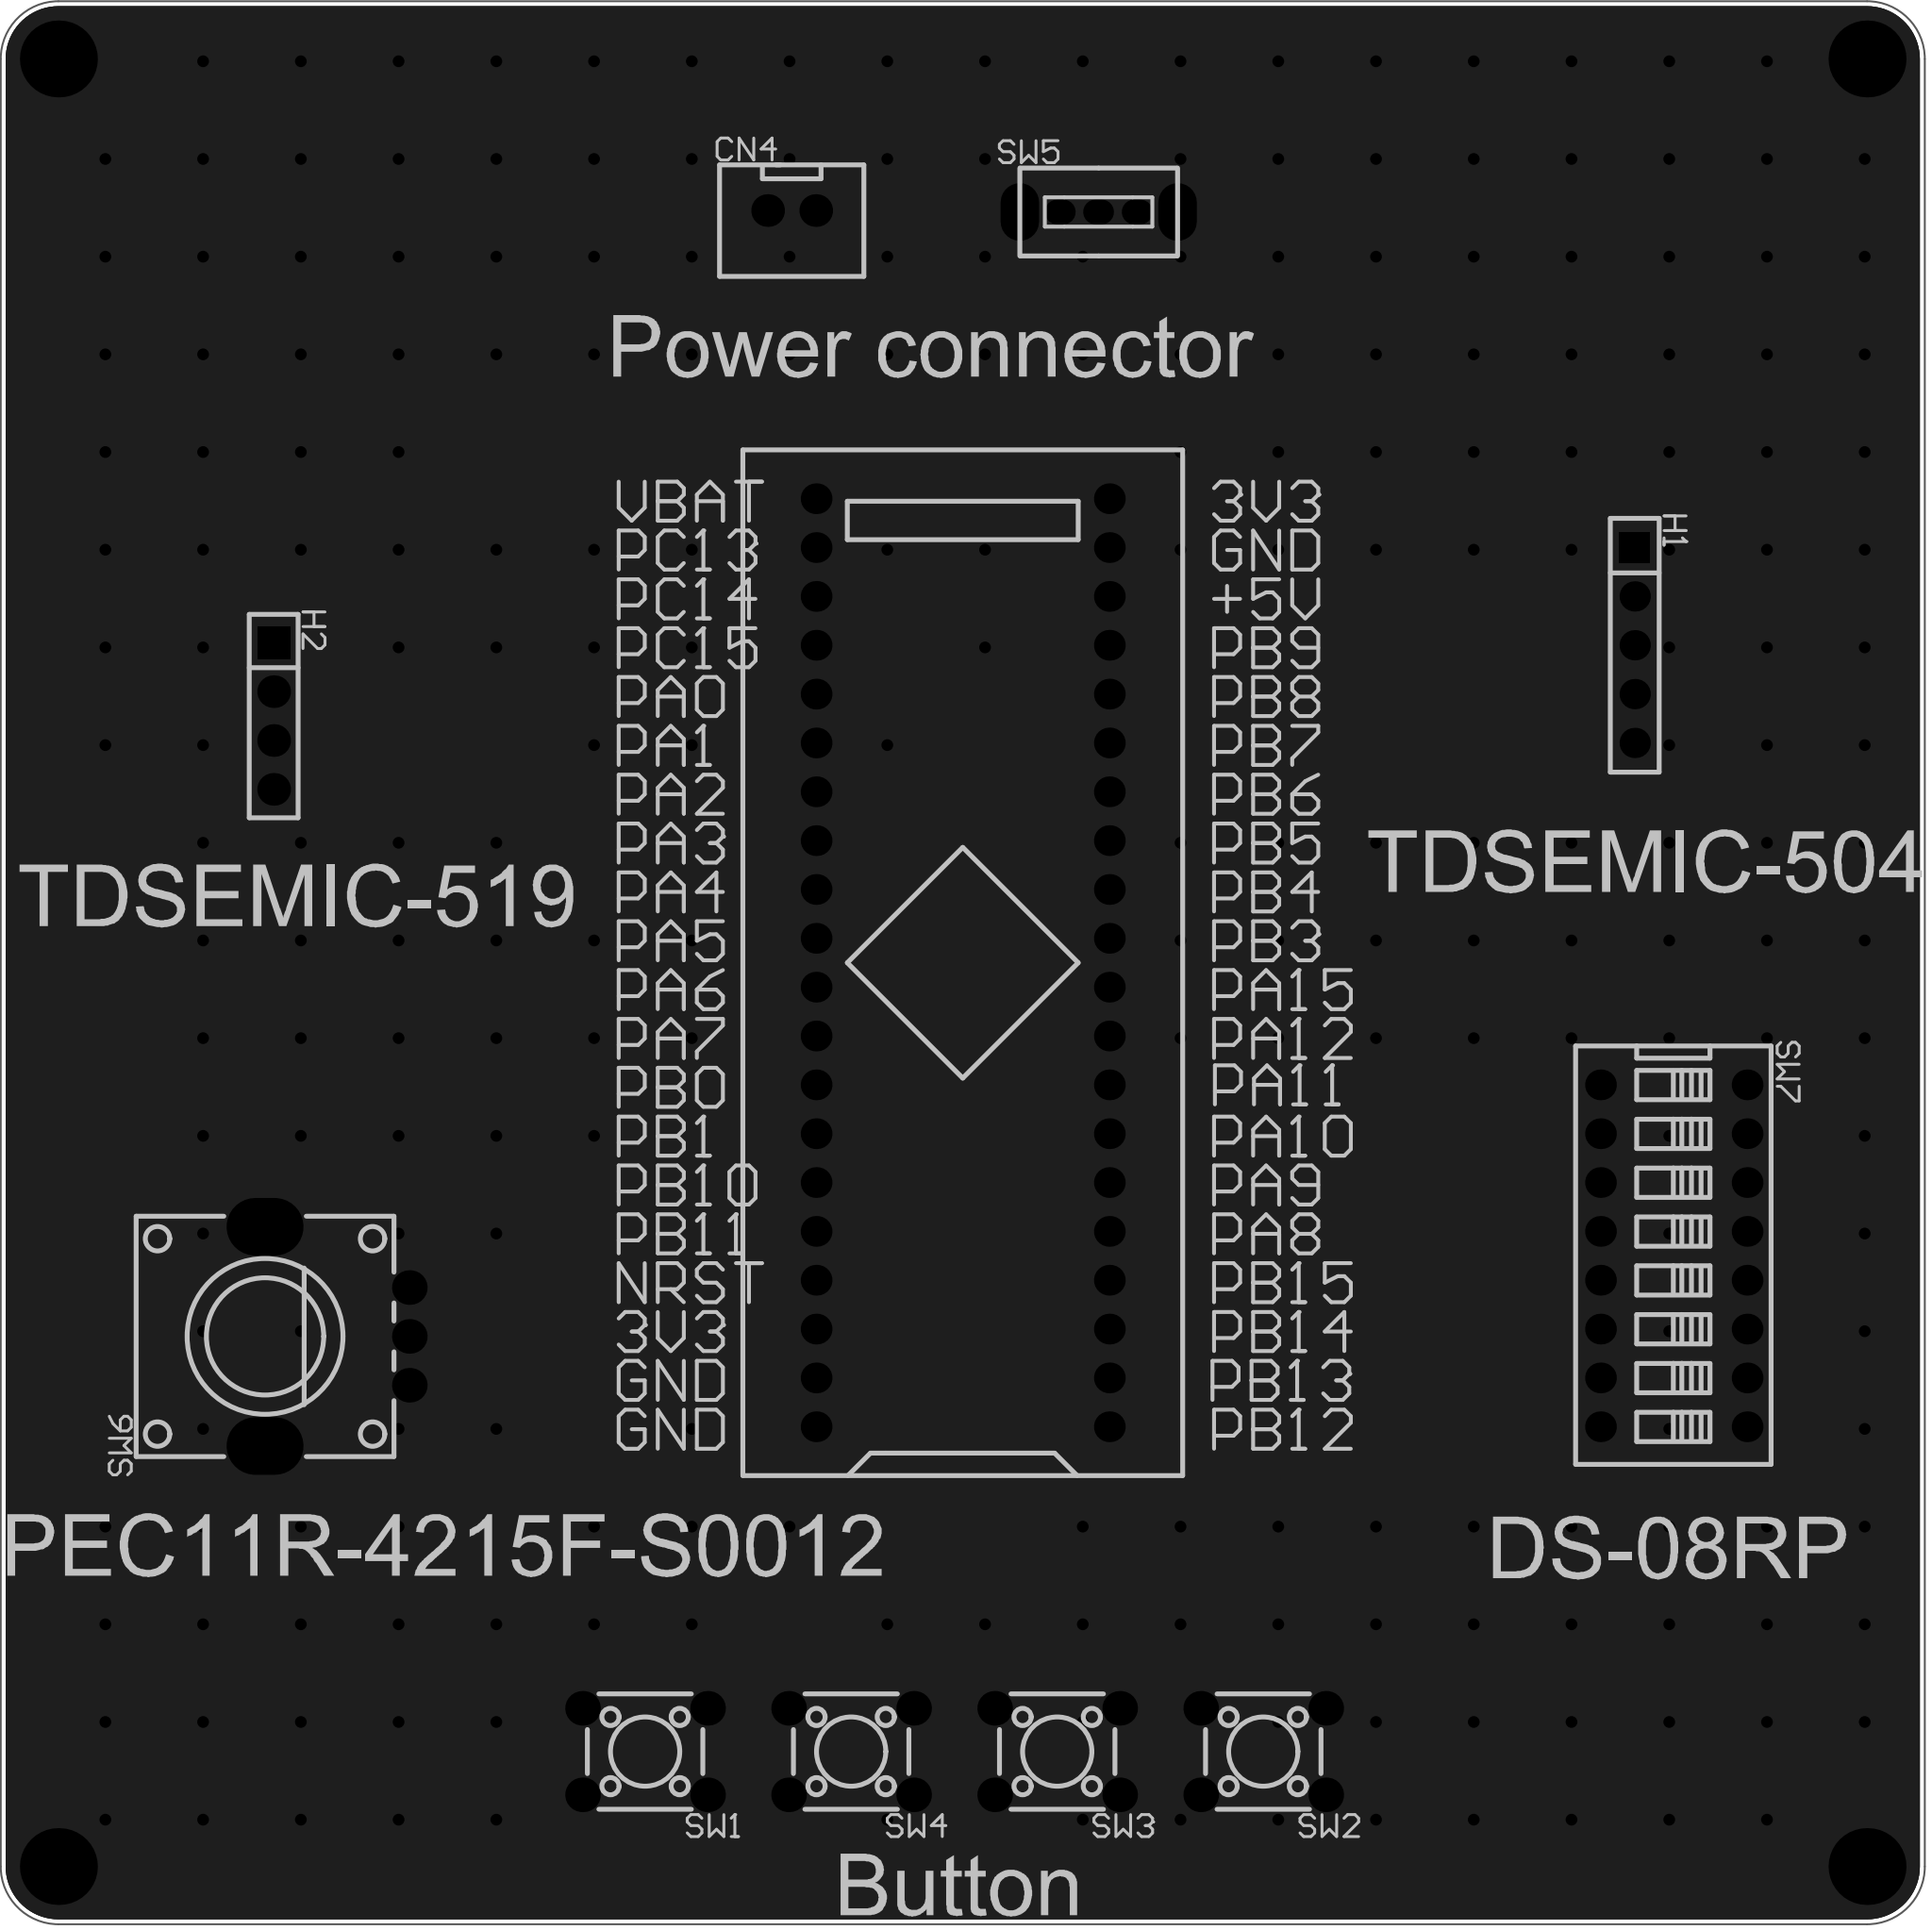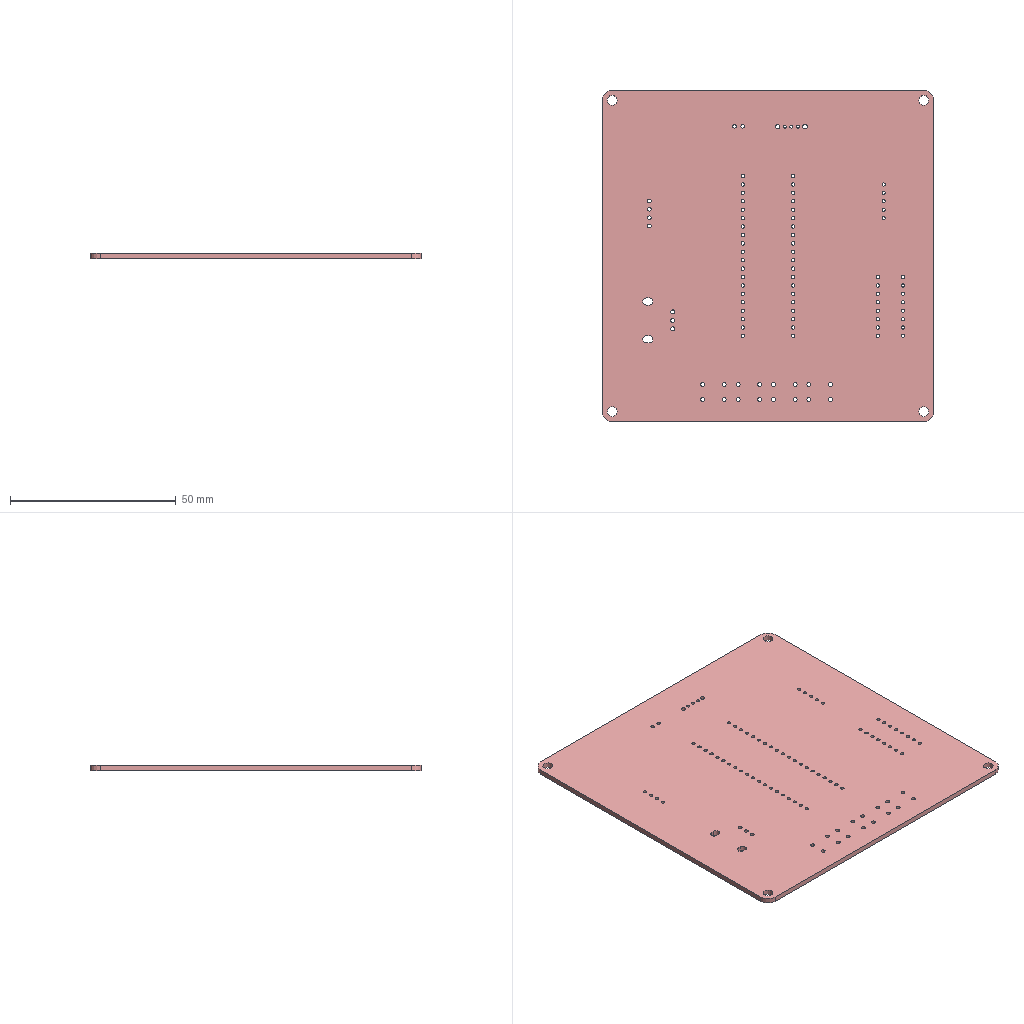Circuit board layout | Altium Designer | box 100 x 100 x 1.6 mm
Layer stack:
# Altium Designer layer stack of  (unit mm; dielectric type: 0 none, 1 core, 2 prepreg, 3 surface material)
index,name,kind,layer,copper_thickness_mm,dielectric_type,dielectric_thickness_mm,dielectric_material,dielectric_constant
0,Top Paste Mask Layer,other,,,,,,
1,Top Silkscreen Layer,other,,,,,,
2,Top Solder Mask Layer,dielectric,,,3,0.01,,3.3
3,Top Layer,copper,Top Layer,0.035,,,,
4,Dielectric1,dielectric,,,3,1.51,FR4,4.5
5,Bottom Layer,copper,Bottom Layer,0.035,,,,
6,Bottom Solder Mask Layer,dielectric,,,3,0.01,,3.3
7,Bottom Silkscreen Layer,other,,,,,,
8,Bottom Paste Mask Layer,other,,,,,,
# drill layer pairs: low layer,high layer
drill_pair,Top Layer,Bottom Layer
Part placement:
Designator,Comment,Layer,Footprint,Center-X(mm),Center-Y(mm),Rotation
U1,STM32F103C8T6-Card,TopLayer,CONN-TH_L53.3-W22.9_STM32F103C8T6-CARD,141.351,130.937,90
SW1,,TopLayer,SW-TH_4P-L6.0-W6.0-P4.50-LS6.5,124.841,89.916,180
SW2,,TopLayer,SW-TH_4P-L6.0-W6.0-P4.50-LS6.5,156.97,89.916,180
SW3,,TopLayer,SW-TH_4P-L6.0-W6.0-P4.50-LS6.5,146.26,89.916,180
SW4,,TopLayer,SW-TH_4P-L6.0-W6.0-P4.50-LS6.5,135.55,89.916,180
CN4,XH2.54*2P_THT,TopLayer,CONN-TH_2P-P2.50-XH2.54-2P,132.461,170.053,0
SW5,,TopLayer,拨动开关,148.417,169.978,0
H1,,TopLayer,HDR-TH_5P-P2.54-V-F,176.276,147.447,270
H2,,TopLayer,HDR-TH_4P-P2.54-V-F,105.537,143.764,270
SW6,PEC11R-4215F-N0024,TopLayer,SW-TH_PEC11R-4215F-N0024,108.839,111.506,90
SW7,DS-08RP,TopLayer,SW-TH_DS-08XP,178.308,115.697,270
Pad and via stacks:
# Altium Designer via and pad stacks of  (unit mm). Each distinct definition once, with the count of objects using it.
# via: kind,start_layer,end_layer,hole_mm,diameter_mm,mode(0 simple;1 top-mid-bottom;2 full stack),diameter_per_layer,count,example_net
# pad: kind,layer,hole_mm,hole_type(0 round;1 square;2 slot),plating,top_size,top_shape(1 round;2 rect;3 octagon;9 rounded rect),mid_size,bottom_size,mode,footprint,size_per_layer,count,example
pad,Multi-Layer,3,0,plated,4x4,1,4x4,4x4,0,,,4,1
pad,Multi-Layer,1,0,plated,1.6x1.6,1,1.6x1.6,1.6x1.6,0,CONN-TH_L53.3-W22.9_STM32F103C8T6-CARD,,40,U1.1
pad,Multi-Layer,1.2,0,plated,1.8x1.8,1,1.8x1.8,1.8x1.8,0,SW-TH_4P-L6.0-W6.0-P4.50-LS6.5,,16,SW1.1
pad,Multi-Layer,1.05,0,plated,1.7x1.7,1,1.7x1.7,1.7x1.7,0,CONN-TH_2P-P2.50-XH2.54-2P,,2,CN4.2
pad,Multi-Layer,0.8992,0,plated,1.6x1.3,1,1.6x1.3,1.6x1.3,0,\u00B2\u00A6\u00B6\u00AF\u00BF\u00AA\u00B9\u00D8,,3,SW5.1
pad,Multi-Layer,1.3,0,plated,3x1.999,1,3x1.999,3x1.999,0,\u00B2\u00A6\u00B6\u00AF\u00BF\u00AA\u00B9\u00D8,,2,SW5.4
pad,Multi-Layer,1.02,0,plated,1.575x1.575,1,1.575x1.575,1.575x1.575,0,HDR-TH_5P-P2.54-V-F,,4,H1.5
pad,Multi-Layer,1.02,0,plated,1.575x1.575,2,1.575x1.575,1.575x1.575,0,HDR-TH_5P-P2.54-V-F,,1,H1.1
pad,Multi-Layer,1.1,0,plated,1.7x1.7,2,1.7x1.7,1.7x1.7,0,HDR-TH_4P-P2.54-V-F,,1,H2.1
pad,Multi-Layer,1.1,0,plated,1.7x1.7,1,1.7x1.7,1.7x1.7,0,HDR-TH_4P-P2.54-V-F,,3,H2.2
pad,Multi-Layer,1.2,0,plated,1.8x1.8,1,1.8x1.8,1.8x1.8,0,SW-TH_PEC11R-4215F-N0024,,3,SW6.A
pad,Multi-Layer,2.2,2,plated,3x4,1,3x4,3x4,0,SW-TH_PEC11R-4215F-N0024,,2,SW6.4
pad,Multi-Layer,1,0,plated,1.6x1.6,1,1.6x1.6,1.6x1.6,0,SW-TH_DS-08XP,,16,SW7.8
via,Top Layer,Bottom Layer,0.3048,0.61,0,,243,GND
Copper pours:
name,layer,net,type(0 solid;1 hatched;2 none)
Bottom Layer-GND,Bottom Layer,GND,0
Top Layer-GND,Top Layer,GND,0
Top Layer-GND 1,Top Layer,GND,0